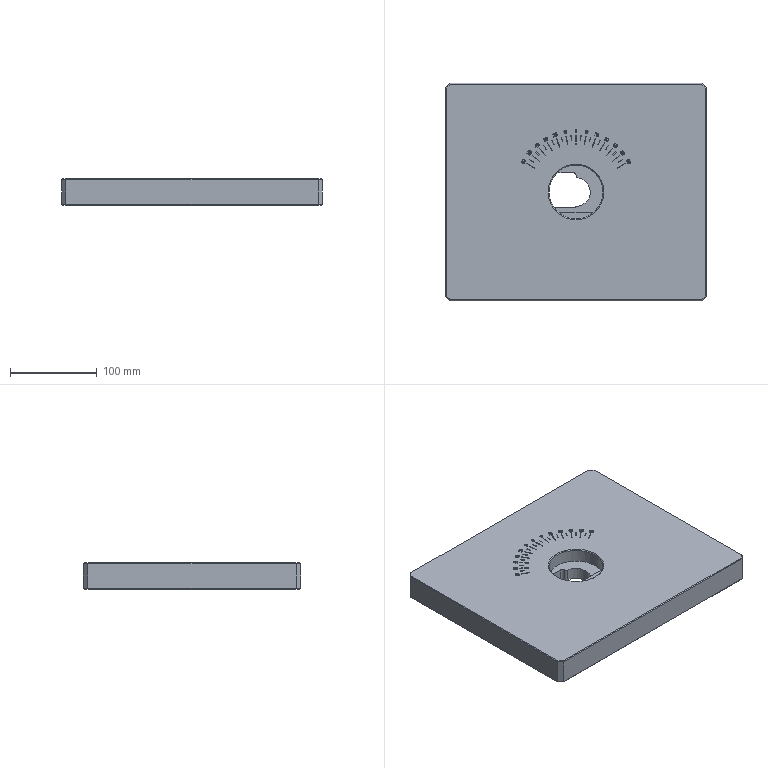Part | 1 solid | 1195 faces | box 300 x 250 x 30 mm | volume 2179035 mm3 | plane 1183 | cylinder 10 | cone 2 | commonest cylinder face diameters 5.2 x7 62.2 x2 33 x1